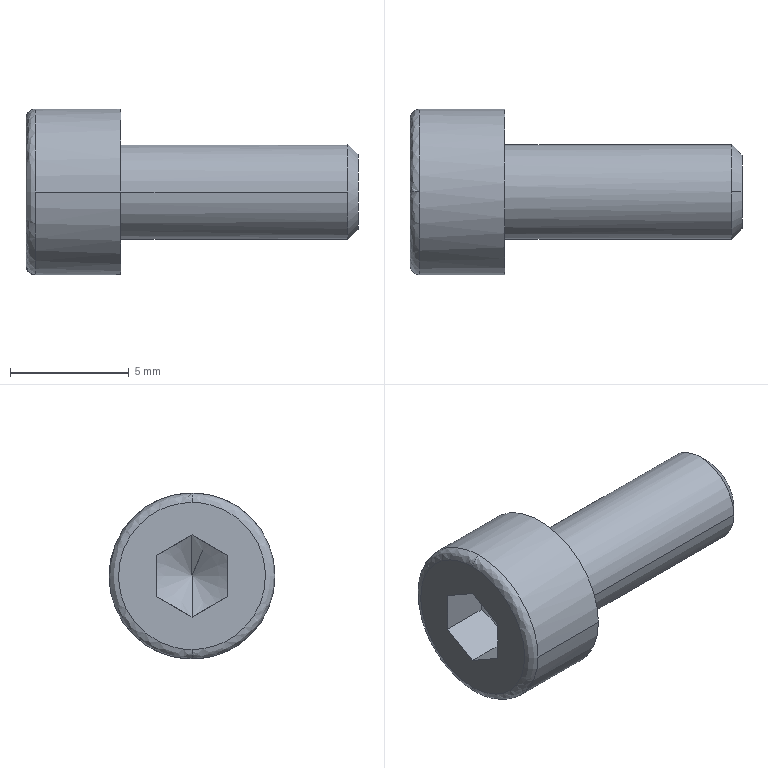Part | SolidWorks | features BaseBody 1 | 1 solid | 19 faces | box 14 x 7 x 7 mm | volume 259.154 mm3 | plane 9 | cylinder 4 | cone 4 | spline 2 | commonest cylinder face diameters 4 x2 7 x2
STEP:
#1=CARTESIAN_POINT('',(-3.6,0.,3.5));
#2=VERTEX_POINT('',#1);
#3=CARTESIAN_POINT('',(-3.6,-3.5,0.));
#4=VERTEX_POINT('',#3);
#5=CARTESIAN_POINT('',(-3.6,0.,0.));
#6=DIRECTION('',(1.,0.,0.));
#7=DIRECTION('',(0.,1.,0.));
#8=AXIS2_PLACEMENT_3D('',#5,#6,#7);
#9=CIRCLE('',#8,3.5);
#10=EDGE_CURVE('',#2,#4,#9,.T.);
#11=ORIENTED_EDGE('',*,*,#10,.F.);
#12=CARTESIAN_POINT('',(-4.,0.,3.1));
#13=VERTEX_POINT('',#12);
#14=CARTESIAN_POINT('',(-3.6,0.,3.1));
#15=DIRECTION('',(0.,-1.,0.));
#16=DIRECTION('',(0.,0.,1.));
#17=AXIS2_PLACEMENT_3D('',#14,#15,#16);
#18=CIRCLE('',#17,0.4);
#19=EDGE_CURVE('',#2,#13,#18,.T.);
#20=ORIENTED_EDGE('',*,*,#19,.T.);
#21=CARTESIAN_POINT('',(-4.,0.,-3.1));
#22=VERTEX_POINT('',#21);
#23=CARTESIAN_POINT('',(-4.,0.,3.1));
#24=CARTESIAN_POINT('',(-4.,-6.2,3.1));
#25=CARTESIAN_POINT('',(-4.,-6.2,-3.1));
#26=CARTESIAN_POINT('',(-4.,0.,-3.1));
#27=(BOUNDED_CURVE()B_SPLINE_CURVE(3,(#23,#24,#25,#26),.UNSPECIFIED.,.F.,.F.)B_SPLINE_CURVE_WITH_KNOTS((4,4),(0.25,0.75),.UNSPECIFIED.)CURVE()GEOMETRIC_REPRESENTATION_ITEM()RATIONAL_B_SPLINE_CURVE((1.,0.3333,0.3333,1.))REPRESENTATION_ITEM(''));
#28=EDGE_CURVE('',#13,#22,#27,.T.);
#29=ORIENTED_EDGE('',*,*,#28,.T.);
#30=CARTESIAN_POINT('',(-3.6,0.,-3.5));
#31=VERTEX_POINT('',#30);
#32=CARTESIAN_POINT('',(-3.6,0.,-3.1));
#33=DIRECTION('',(0.,1.,0.));
#34=DIRECTION('',(0.,0.,-1.));
#35=AXIS2_PLACEMENT_3D('',#32,#33,#34);
#36=CIRCLE('',#35,0.4);
#37=EDGE_CURVE('',#31,#22,#36,.T.);
#38=ORIENTED_EDGE('',*,*,#37,.F.);
#39=CARTESIAN_POINT('',(-3.6,0.,0.));
#40=DIRECTION('',(1.,0.,0.));
#41=DIRECTION('',(0.,1.,0.));
#42=AXIS2_PLACEMENT_3D('',#39,#40,#41);
#43=CIRCLE('',#42,3.5);
#44=EDGE_CURVE('',#4,#31,#43,.T.);
#45=ORIENTED_EDGE('',*,*,#44,.F.);
#46=EDGE_LOOP('',(#11,#20,#29,#38,#45));
#47=FACE_OUTER_BOUND('',#46,.T.);
#48=CARTESIAN_POINT('',(-3.6,0.,3.5));
#49=CARTESIAN_POINT('',(-3.6,-7.,3.5));
#50=CARTESIAN_POINT('',(-3.6,-7.,-3.5));
#51=CARTESIAN_POINT('',(-3.6,0.,-3.5));
#52=CARTESIAN_POINT('',(-3.834,0.,3.5));
#53=CARTESIAN_POINT('',(-3.834,-7.,3.5));
#54=CARTESIAN_POINT('',(-3.834,-7.,-3.5));
#55=CARTESIAN_POINT('',(-3.834,0.,-3.5));
#56=CARTESIAN_POINT('',(-4.,0.,3.334));
#57=CARTESIAN_POINT('',(-4.,-6.669,3.334));
#58=CARTESIAN_POINT('',(-4.,-6.669,-3.334));
#59=CARTESIAN_POINT('',(-4.,0.,-3.334));
#60=CARTESIAN_POINT('',(-4.,0.,3.1));
#61=CARTESIAN_POINT('',(-4.,-6.2,3.1));
#62=CARTESIAN_POINT('',(-4.,-6.2,-3.1));
#63=CARTESIAN_POINT('',(-4.,0.,-3.1));
#64=(BOUNDED_SURFACE()B_SPLINE_SURFACE(3,3,((#48,#49,#50,#51),(#52,#53,#54,#55),(#56,#57,#58,#59),(#60,#61,#62,#63)),.UNSPECIFIED.,.F.,.F.,.F.)B_SPLINE_SURFACE_WITH_KNOTS((4,4),(4,4),(0.,1.),(0.,1.),.UNSPECIFIED.)GEOMETRIC_REPRESENTATION_ITEM()RATIONAL_B_SPLINE_SURFACE(((1.,0.3333,0.3333,1.),(0.8047,0.2682,0.2682,0.8047),(0.8047,0.2682,0.2682,0.8047),(1.,0.3333,0.3333,1.)))REPRESENTATION_ITEM('')SURFACE());
#65=ADVANCED_FACE('',(#47),#64,.T.);
#66=CARTESIAN_POINT('',(0.,2.,0.));
#67=VERTEX_POINT('',#66);
#68=CARTESIAN_POINT('',(0.,-2.,0.));
#69=VERTEX_POINT('',#68);
#70=CARTESIAN_POINT('',(0.,0.,0.));
#71=DIRECTION('',(1.,0.,0.));
#72=DIRECTION('',(0.,1.,0.));
#73=AXIS2_PLACEMENT_3D('',#70,#71,#72);
#74=CIRCLE('',#73,2.);
#75=EDGE_CURVE('',#67,#69,#74,.T.);
#76=ORIENTED_EDGE('',*,*,#75,.T.);
#77=CARTESIAN_POINT('',(9.571,-2.,0.));
#78=VERTEX_POINT('',#77);
#79=CARTESIAN_POINT('',(5.875,-2.,0.));
#80=DIRECTION('',(1.,0.,0.));
#81=VECTOR('',#80,1000.);
#82=LINE('',#79,#81);
#83=EDGE_CURVE('',#69,#78,#82,.T.);
#84=ORIENTED_EDGE('',*,*,#83,.T.);
#85=CARTESIAN_POINT('',(9.571,0.,2.));
#86=VERTEX_POINT('',#85);
#87=CARTESIAN_POINT('',(9.571,0.,0.));
#88=DIRECTION('',(-1.,0.,0.));
#89=DIRECTION('',(0.,1.,0.));
#90=AXIS2_PLACEMENT_3D('',#87,#88,#89);
#91=CIRCLE('',#90,2.);
#92=EDGE_CURVE('',#78,#86,#91,.T.);
#93=ORIENTED_EDGE('',*,*,#92,.T.);
#94=CARTESIAN_POINT('',(9.571,2.,0.));
#95=VERTEX_POINT('',#94);
#96=CARTESIAN_POINT('',(9.571,0.,0.));
#97=DIRECTION('',(-1.,0.,0.));
#98=DIRECTION('',(0.,1.,0.));
#99=AXIS2_PLACEMENT_3D('',#96,#97,#98);
#100=CIRCLE('',#99,2.);
#101=EDGE_CURVE('',#86,#95,#100,.T.);
#102=ORIENTED_EDGE('',*,*,#101,.T.);
#103=CARTESIAN_POINT('',(5.875,2.,0.));
#104=DIRECTION('',(1.,0.,0.));
#105=VECTOR('',#104,1000.);
#106=LINE('',#103,#105);
#107=EDGE_CURVE('',#67,#95,#106,.T.);
#108=ORIENTED_EDGE('',*,*,#107,.F.);
#109=EDGE_LOOP('',(#76,#84,#93,#102,#108));
#110=FACE_OUTER_BOUND('',#109,.T.);
#111=CARTESIAN_POINT('',(5.875,0.,0.));
#112=DIRECTION('',(1.,0.,0.));
#113=DIRECTION('',(0.,1.,0.));
#114=AXIS2_PLACEMENT_3D('',#111,#112,#113);
#115=CYLINDRICAL_SURFACE('',#114,2.);
#116=ADVANCED_FACE('',(#110),#115,.T.);
#117=CARTESIAN_POINT('',(10.,0.,1.571));
#118=VERTEX_POINT('',#117);
#119=CARTESIAN_POINT('',(10.,0.,-1.571));
#120=VERTEX_POINT('',#119);
#121=CARTESIAN_POINT('',(10.,0.,0.));
#122=DIRECTION('',(-1.,0.,0.));
#123=DIRECTION('',(0.,0.,1.));
#124=AXIS2_PLACEMENT_3D('',#121,#122,#123);
#125=CIRCLE('',#124,1.571);
#126=EDGE_CURVE('',#118,#120,#125,.T.);
#127=ORIENTED_EDGE('',*,*,#126,.T.);
#128=CARTESIAN_POINT('',(9.571,0.,-2.));
#129=VERTEX_POINT('',#128);
#130=CARTESIAN_POINT('',(9.571,0.,-2.));
#131=DIRECTION('',(-0.7071,0.,-0.7071));
#132=VECTOR('',#131,1000.);
#133=LINE('',#130,#132);
#134=EDGE_CURVE('',#120,#129,#133,.T.);
#135=ORIENTED_EDGE('',*,*,#134,.T.);
#136=CARTESIAN_POINT('',(9.571,0.,0.));
#137=DIRECTION('',(-1.,0.,0.));
#138=DIRECTION('',(0.,1.,0.));
#139=AXIS2_PLACEMENT_3D('',#136,#137,#138);
#140=CIRCLE('',#139,2.);
#141=EDGE_CURVE('',#95,#129,#140,.T.);
#142=ORIENTED_EDGE('',*,*,#141,.F.);
#143=ORIENTED_EDGE('',*,*,#101,.F.);
#144=CARTESIAN_POINT('',(9.571,0.,2.));
#145=DIRECTION('',(-0.7071,0.,0.7071));
#146=VECTOR('',#145,1000.);
#147=LINE('',#144,#146);
#148=EDGE_CURVE('',#118,#86,#147,.T.);
#149=ORIENTED_EDGE('',*,*,#148,.F.);
#150=EDGE_LOOP('',(#127,#135,#142,#143,#149));
#151=FACE_OUTER_BOUND('',#150,.T.);
#152=CARTESIAN_POINT('',(9.571,0.,0.));
#153=DIRECTION('',(-1.,0.,0.));
#154=DIRECTION('',(0.,0.,1.));
#155=AXIS2_PLACEMENT_3D('',#152,#153,#154);
#156=CONICAL_SURFACE('',#155,2.,0.7854);
#157=ADVANCED_FACE('',(#151),#156,.T.);
#158=CARTESIAN_POINT('',(-3.6,3.5,0.));
#159=VERTEX_POINT('',#158);
#160=CARTESIAN_POINT('',(-3.6,0.,0.));
#161=DIRECTION('',(1.,0.,0.));
#162=DIRECTION('',(0.,1.,0.));
#163=AXIS2_PLACEMENT_3D('',#160,#161,#162);
#164=CIRCLE('',#163,3.5);
#165=EDGE_CURVE('',#159,#2,#164,.T.);
#166=ORIENTED_EDGE('',*,*,#165,.T.);
#167=ORIENTED_EDGE('',*,*,#10,.T.);
#168=CARTESIAN_POINT('',(0.,-3.5,0.));
#169=VERTEX_POINT('',#168);
#170=CARTESIAN_POINT('',(-2.,-3.5,0.));
#171=DIRECTION('',(1.,0.,0.));
#172=VECTOR('',#171,1000.);
#173=LINE('',#170,#172);
#174=EDGE_CURVE('',#4,#169,#173,.T.);
#175=ORIENTED_EDGE('',*,*,#174,.T.);
#176=CARTESIAN_POINT('',(0.,3.5,0.));
#177=VERTEX_POINT('',#176);
#178=CARTESIAN_POINT('',(0.,0.,0.));
#179=DIRECTION('',(1.,0.,0.));
#180=DIRECTION('',(0.,1.,0.));
#181=AXIS2_PLACEMENT_3D('',#178,#179,#180);
#182=CIRCLE('',#181,3.5);
#183=EDGE_CURVE('',#177,#169,#182,.T.);
#184=ORIENTED_EDGE('',*,*,#183,.F.);
#185=CARTESIAN_POINT('',(-2.,3.5,0.));
#186=DIRECTION('',(1.,0.,0.));
#187=VECTOR('',#186,1000.);
#188=LINE('',#185,#187);
#189=EDGE_CURVE('',#159,#177,#188,.T.);
#190=ORIENTED_EDGE('',*,*,#189,.F.);
#191=EDGE_LOOP('',(#166,#167,#175,#184,#190));
#192=FACE_OUTER_BOUND('',#191,.T.);
#193=CARTESIAN_POINT('',(-2.,0.,0.));
#194=DIRECTION('',(1.,0.,0.));
#195=DIRECTION('',(0.,1.,0.));
#196=AXIS2_PLACEMENT_3D('',#193,#194,#195);
#197=CYLINDRICAL_SURFACE('',#196,3.5);
#198=ADVANCED_FACE('',(#192),#197,.T.);
#199=CARTESIAN_POINT('',(-1.,0.,0.));
#200=VERTEX_POINT('',#199);
#201=CARTESIAN_POINT('',(-2.,0.000000012,1.732));
#202=VERTEX_POINT('',#201);
#203=CARTESIAN_POINT('',(-2.006,0.,1.742));
#204=DIRECTION('',(-0.5,0.,0.866));
#205=VECTOR('',#204,1000.);
#206=LINE('',#203,#205);
#207=EDGE_CURVE('',#200,#202,#206,.T.);
#208=ORIENTED_EDGE('',*,*,#207,.F.);
#209=CARTESIAN_POINT('',(-2.,-0.000000052,-1.732));
#210=VERTEX_POINT('',#209);
#211=CARTESIAN_POINT('',(-2.006,0.,-1.742));
#212=DIRECTION('',(-0.5,0.,-0.866));
#213=VECTOR('',#212,1000.);
#214=LINE('',#211,#213);
#215=EDGE_CURVE('',#200,#210,#214,.T.);
#216=ORIENTED_EDGE('',*,*,#215,.T.);
#217=CARTESIAN_POINT('',(-2.,-1.5,-0.866));
#218=VERTEX_POINT('',#217);
#219=CARTESIAN_POINT('',(-2.,-1.5,-0.866));
#220=CARTESIAN_POINT('',(-1.918,-1.255,-1.007));
#221=CARTESIAN_POINT('',(-1.866,-1.006,-1.151));
#222=CARTESIAN_POINT('',(-1.866,-0.4964,-1.445));
#223=CARTESIAN_POINT('',(-1.918,-0.2452,-1.59));
#224=CARTESIAN_POINT('',(-2.,-0.000000052,-1.732));
#225=B_SPLINE_CURVE_WITH_KNOTS('',3,(#219,#220,#221,#222,#223,#224),.UNSPECIFIED.,.F.,.F.,(4,2,4),(0.,0.0008746,0.001749),.UNSPECIFIED.);
#226=EDGE_CURVE('',#218,#210,#225,.T.);
#227=ORIENTED_EDGE('',*,*,#226,.F.);
#228=CARTESIAN_POINT('',(-2.,-1.5,0.866));
#229=VERTEX_POINT('',#228);
#230=CARTESIAN_POINT('',(-2.,-1.5,0.866));
#231=CARTESIAN_POINT('',(-1.918,-1.5,0.5832));
#232=CARTESIAN_POINT('',(-1.866,-1.5,0.2962));
#233=CARTESIAN_POINT('',(-1.866,-1.5,-0.2929));
#234=CARTESIAN_POINT('',(-1.918,-1.5,-0.5829));
#235=CARTESIAN_POINT('',(-2.,-1.5,-0.866));
#236=B_SPLINE_CURVE_WITH_KNOTS('',3,(#230,#231,#232,#233,#234,#235),.UNSPECIFIED.,.F.,.F.,(4,2,4),(0.,0.0008746,0.001749),.UNSPECIFIED.);
#237=EDGE_CURVE('',#229,#218,#236,.T.);
#238=ORIENTED_EDGE('',*,*,#237,.F.);
#239=CARTESIAN_POINT('',(-2.,0.000000012,1.732));
#240=CARTESIAN_POINT('',(-1.918,-0.2449,1.591));
#241=CARTESIAN_POINT('',(-1.866,-0.4935,1.447));
#242=CARTESIAN_POINT('',(-1.866,-1.004,1.153));
#243=CARTESIAN_POINT('',(-1.918,-1.255,1.008));
#244=CARTESIAN_POINT('',(-2.,-1.5,0.866));
#245=B_SPLINE_CURVE_WITH_KNOTS('',3,(#239,#240,#241,#242,#243,#244),.UNSPECIFIED.,.F.,.F.,(4,2,4),(0.,0.0008746,0.001749),.UNSPECIFIED.);
#246=EDGE_CURVE('',#202,#229,#245,.T.);
#247=ORIENTED_EDGE('',*,*,#246,.F.);
#248=EDGE_LOOP('',(#208,#216,#227,#238,#247));
#249=FACE_OUTER_BOUND('',#248,.T.);
#250=CARTESIAN_POINT('',(-2.006,0.,0.));
#251=DIRECTION('',(-1.,0.,0.));
#252=DIRECTION('',(0.,0.,1.));
#253=AXIS2_PLACEMENT_3D('',#250,#251,#252);
#254=CONICAL_SURFACE('',#253,1.742,1.047);
#255=ADVANCED_FACE('',(#249),#254,.F.);
#256=ORIENTED_EDGE('',*,*,#83,.F.);
#257=CARTESIAN_POINT('',(0.,0.,0.));
#258=DIRECTION('',(1.,0.,0.));
#259=DIRECTION('',(0.,1.,0.));
#260=AXIS2_PLACEMENT_3D('',#257,#258,#259);
#261=CIRCLE('',#260,2.);
#262=EDGE_CURVE('',#69,#67,#261,.T.);
#263=ORIENTED_EDGE('',*,*,#262,.T.);
#264=ORIENTED_EDGE('',*,*,#107,.T.);
#265=ORIENTED_EDGE('',*,*,#141,.T.);
#266=CARTESIAN_POINT('',(9.571,0.,0.));
#267=DIRECTION('',(-1.,0.,0.));
#268=DIRECTION('',(0.,1.,0.));
#269=AXIS2_PLACEMENT_3D('',#266,#267,#268);
#270=CIRCLE('',#269,2.);
#271=EDGE_CURVE('',#129,#78,#270,.T.);
#272=ORIENTED_EDGE('',*,*,#271,.T.);
#273=EDGE_LOOP('',(#256,#263,#264,#265,#272));
#274=FACE_OUTER_BOUND('',#273,.T.);
#275=CARTESIAN_POINT('',(5.875,0.,0.));
#276=DIRECTION('',(1.,0.,0.));
#277=DIRECTION('',(0.,1.,0.));
#278=AXIS2_PLACEMENT_3D('',#275,#276,#277);
#279=CYLINDRICAL_SURFACE('',#278,2.);
#280=ADVANCED_FACE('',(#274),#279,.T.);
#281=ORIENTED_EDGE('',*,*,#134,.F.);
#282=CARTESIAN_POINT('',(10.,0.,0.));
#283=DIRECTION('',(-1.,0.,0.));
#284=DIRECTION('',(0.,0.,1.));
#285=AXIS2_PLACEMENT_3D('',#282,#283,#284);
#286=CIRCLE('',#285,1.571);
#287=EDGE_CURVE('',#120,#118,#286,.T.);
#288=ORIENTED_EDGE('',*,*,#287,.T.);
#289=ORIENTED_EDGE('',*,*,#148,.T.);
#290=ORIENTED_EDGE('',*,*,#92,.F.);
#291=ORIENTED_EDGE('',*,*,#271,.F.);
#292=EDGE_LOOP('',(#281,#288,#289,#290,#291));
#293=FACE_OUTER_BOUND('',#292,.T.);
#294=CARTESIAN_POINT('',(9.571,0.,0.));
#295=DIRECTION('',(-1.,0.,0.));
#296=DIRECTION('',(0.,0.,1.));
#297=AXIS2_PLACEMENT_3D('',#294,#295,#296);
#298=CONICAL_SURFACE('',#297,2.,0.7854);
#299=ADVANCED_FACE('',(#293),#298,.T.);
#300=ORIENTED_EDGE('',*,*,#75,.F.);
#301=ORIENTED_EDGE('',*,*,#262,.F.);
#302=EDGE_LOOP('',(#300,#301));
#303=FACE_BOUND('',#302,.T.);
#304=ORIENTED_EDGE('',*,*,#183,.T.);
#305=CARTESIAN_POINT('',(0.,0.,0.));
#306=DIRECTION('',(1.,0.,0.));
#307=DIRECTION('',(0.,1.,0.));
#308=AXIS2_PLACEMENT_3D('',#305,#306,#307);
#309=CIRCLE('',#308,3.5);
#310=EDGE_CURVE('',#169,#177,#309,.T.);
#311=ORIENTED_EDGE('',*,*,#310,.T.);
#312=EDGE_LOOP('',(#304,#311));
#313=FACE_OUTER_BOUND('',#312,.T.);
#314=CARTESIAN_POINT('',(0.,2.75,0.));
#315=DIRECTION('',(1.,0.,0.));
#316=DIRECTION('',(0.,0.,-1.));
#317=AXIS2_PLACEMENT_3D('',#314,#315,#316);
#318=PLANE('',#317);
#319=ADVANCED_FACE('',(#303,#313),#318,.T.);
#320=ORIENTED_EDGE('',*,*,#126,.F.);
#321=ORIENTED_EDGE('',*,*,#287,.F.);
#322=EDGE_LOOP('',(#320,#321));
#323=FACE_OUTER_BOUND('',#322,.T.);
#324=CARTESIAN_POINT('',(10.,1.,0.));
#325=DIRECTION('',(1.,0.,0.));
#326=DIRECTION('',(0.,0.,-1.));
#327=AXIS2_PLACEMENT_3D('',#324,#325,#326);
#328=PLANE('',#327);
#329=ADVANCED_FACE('',(#323),#328,.T.);
#330=ORIENTED_EDGE('',*,*,#174,.F.);
#331=ORIENTED_EDGE('',*,*,#44,.T.);
#332=CARTESIAN_POINT('',(-3.6,0.,0.));
#333=DIRECTION('',(1.,0.,0.));
#334=DIRECTION('',(0.,1.,0.));
#335=AXIS2_PLACEMENT_3D('',#332,#333,#334);
#336=CIRCLE('',#335,3.5);
#337=EDGE_CURVE('',#31,#159,#336,.T.);
#338=ORIENTED_EDGE('',*,*,#337,.T.);
#339=ORIENTED_EDGE('',*,*,#189,.T.);
#340=ORIENTED_EDGE('',*,*,#310,.F.);
#341=EDGE_LOOP('',(#330,#331,#338,#339,#340));
#342=FACE_OUTER_BOUND('',#341,.T.);
#343=CARTESIAN_POINT('',(-2.,0.,0.));
#344=DIRECTION('',(1.,0.,0.));
#345=DIRECTION('',(0.,1.,0.));
#346=AXIS2_PLACEMENT_3D('',#343,#344,#345);
#347=CYLINDRICAL_SURFACE('',#346,3.5);
#348=ADVANCED_FACE('',(#342),#347,.T.);
#349=ORIENTED_EDGE('',*,*,#19,.F.);
#350=ORIENTED_EDGE('',*,*,#165,.F.);
#351=ORIENTED_EDGE('',*,*,#337,.F.);
#352=ORIENTED_EDGE('',*,*,#37,.T.);
#353=CARTESIAN_POINT('',(-4.,0.,-3.1));
#354=CARTESIAN_POINT('',(-4.,6.2,-3.1));
#355=CARTESIAN_POINT('',(-4.,6.2,3.1));
#356=CARTESIAN_POINT('',(-4.,0.,3.1));
#357=(BOUNDED_CURVE()B_SPLINE_CURVE(3,(#353,#354,#355,#356),.UNSPECIFIED.,.F.,.F.)B_SPLINE_CURVE_WITH_KNOTS((4,4),(0.75,1.25),.UNSPECIFIED.)CURVE()GEOMETRIC_REPRESENTATION_ITEM()RATIONAL_B_SPLINE_CURVE((1.,0.3333,0.3333,1.))REPRESENTATION_ITEM(''));
#358=EDGE_CURVE('',#22,#13,#357,.T.);
#359=ORIENTED_EDGE('',*,*,#358,.T.);
#360=EDGE_LOOP('',(#349,#350,#351,#352,#359));
#361=FACE_OUTER_BOUND('',#360,.T.);
#362=CARTESIAN_POINT('',(-3.6,0.,-3.5));
#363=CARTESIAN_POINT('',(-3.6,7.,-3.5));
#364=CARTESIAN_POINT('',(-3.6,7.,3.5));
#365=CARTESIAN_POINT('',(-3.6,0.,3.5));
#366=CARTESIAN_POINT('',(-3.834,0.,-3.5));
#367=CARTESIAN_POINT('',(-3.834,7.,-3.5));
#368=CARTESIAN_POINT('',(-3.834,7.,3.5));
#369=CARTESIAN_POINT('',(-3.834,0.,3.5));
#370=CARTESIAN_POINT('',(-4.,0.,-3.334));
#371=CARTESIAN_POINT('',(-4.,6.669,-3.334));
#372=CARTESIAN_POINT('',(-4.,6.669,3.334));
#373=CARTESIAN_POINT('',(-4.,0.,3.334));
#374=CARTESIAN_POINT('',(-4.,0.,-3.1));
#375=CARTESIAN_POINT('',(-4.,6.2,-3.1));
#376=CARTESIAN_POINT('',(-4.,6.2,3.1));
#377=CARTESIAN_POINT('',(-4.,0.,3.1));
#378=(BOUNDED_SURFACE()B_SPLINE_SURFACE(3,3,((#362,#363,#364,#365),(#366,#367,#368,#369),(#370,#371,#372,#373),(#374,#375,#376,#377)),.UNSPECIFIED.,.F.,.F.,.F.)B_SPLINE_SURFACE_WITH_KNOTS((4,4),(4,4),(0.,1.),(0.,1.),.UNSPECIFIED.)GEOMETRIC_REPRESENTATION_ITEM()RATIONAL_B_SPLINE_SURFACE(((1.,0.3333,0.3333,1.),(0.8047,0.2682,0.2682,0.8047),(0.8047,0.2682,0.2682,0.8047),(1.,0.3333,0.3333,1.)))REPRESENTATION_ITEM('')SURFACE());
#379=ADVANCED_FACE('',(#361),#378,.T.);
#380=CARTESIAN_POINT('',(-4.,-1.5,-0.866));
#381=VERTEX_POINT('',#380);
#382=CARTESIAN_POINT('',(-4.,0.,-1.732));
#383=VERTEX_POINT('',#382);
#384=CARTESIAN_POINT('',(-4.,0.,-1.732));
#385=DIRECTION('',(0.,0.866,-0.5));
#386=VECTOR('',#385,1000.);
#387=LINE('',#384,#386);
#388=EDGE_CURVE('',#381,#383,#387,.T.);
#389=ORIENTED_EDGE('',*,*,#388,.T.);
#390=CARTESIAN_POINT('',(-4.,1.5,-0.866));
#391=VERTEX_POINT('',#390);
#392=CARTESIAN_POINT('',(-4.,0.,-1.732));
#393=DIRECTION('',(0.,0.866,0.5));
#394=VECTOR('',#393,1000.);
#395=LINE('',#392,#394);
#396=EDGE_CURVE('',#383,#391,#395,.T.);
#397=ORIENTED_EDGE('',*,*,#396,.T.);
#398=CARTESIAN_POINT('',(-4.,1.5,0.866));
#399=VERTEX_POINT('',#398);
#400=CARTESIAN_POINT('',(-4.,1.5,0.866));
#401=DIRECTION('',(0.,0.,1.));
#402=VECTOR('',#401,1000.);
#403=LINE('',#400,#402);
#404=EDGE_CURVE('',#391,#399,#403,.T.);
#405=ORIENTED_EDGE('',*,*,#404,.T.);
#406=CARTESIAN_POINT('',(-4.,0.,1.732));
#407=VERTEX_POINT('',#406);
#408=CARTESIAN_POINT('',(-4.,0.,1.732));
#409=DIRECTION('',(0.,-0.866,0.5));
#410=VECTOR('',#409,1000.);
#411=LINE('',#408,#410);
#412=EDGE_CURVE('',#399,#407,#411,.T.);
#413=ORIENTED_EDGE('',*,*,#412,.T.);
#414=CARTESIAN_POINT('',(-4.,-1.5,0.866));
#415=VERTEX_POINT('',#414);
#416=CARTESIAN_POINT('',(-4.,-1.5,0.866));
#417=DIRECTION('',(0.,-0.866,-0.5));
#418=VECTOR('',#417,1000.);
#419=LINE('',#416,#418);
#420=EDGE_CURVE('',#407,#415,#419,.T.);
#421=ORIENTED_EDGE('',*,*,#420,.T.);
#422=CARTESIAN_POINT('',(-4.,-1.5,-0.866));
#423=DIRECTION('',(0.,0.,-1.));
#424=VECTOR('',#423,1000.);
#425=LINE('',#422,#424);
#426=EDGE_CURVE('',#415,#381,#425,.T.);
#427=ORIENTED_EDGE('',*,*,#426,.T.);
#428=EDGE_LOOP('',(#389,#397,#405,#413,#421,#427));
#429=FACE_BOUND('',#428,.T.);
#430=ORIENTED_EDGE('',*,*,#358,.F.);
#431=ORIENTED_EDGE('',*,*,#28,.F.);
#432=EDGE_LOOP('',(#430,#431));
#433=FACE_OUTER_BOUND('',#432,.T.);
#434=CARTESIAN_POINT('',(-4.,2.616,0.));
#435=DIRECTION('',(-1.,0.,0.));
#436=DIRECTION('',(0.,0.,1.));
#437=AXIS2_PLACEMENT_3D('',#434,#435,#436);
#438=PLANE('',#437);
#439=ADVANCED_FACE('',(#429,#433),#438,.T.);
#440=CARTESIAN_POINT('',(-2.,1.5,-0.866));
#441=VERTEX_POINT('',#440);
#442=CARTESIAN_POINT('',(-4.,1.5,-0.866));
#443=DIRECTION('',(1.,0.,0.));
#444=VECTOR('',#443,1000.);
#445=LINE('',#442,#444);
#446=EDGE_CURVE('',#391,#441,#445,.T.);
#447=ORIENTED_EDGE('',*,*,#446,.F.);
#448=ORIENTED_EDGE('',*,*,#396,.F.);
#449=CARTESIAN_POINT('',(-4.,0.,-1.732));
#450=DIRECTION('',(-1.,0.,0.));
#451=VECTOR('',#450,1000.);
#452=LINE('',#449,#451);
#453=EDGE_CURVE('',#210,#383,#452,.T.);
#454=ORIENTED_EDGE('',*,*,#453,.F.);
#455=CARTESIAN_POINT('',(-2.,1.5,-0.866));
#456=CARTESIAN_POINT('',(-1.918,1.255,-1.007));
#457=CARTESIAN_POINT('',(-1.866,1.006,-1.151));
#458=CARTESIAN_POINT('',(-1.866,0.4964,-1.445));
#459=CARTESIAN_POINT('',(-1.918,0.2452,-1.59));
#460=CARTESIAN_POINT('',(-2.,-0.000000052,-1.732));
#461=B_SPLINE_CURVE_WITH_KNOTS('',3,(#455,#456,#457,#458,#459,#460),.UNSPECIFIED.,.F.,.F.,(4,2,4),(0.,0.0008746,0.001749),.UNSPECIFIED.);
#462=EDGE_CURVE('',#441,#210,#461,.T.);
#463=ORIENTED_EDGE('',*,*,#462,.F.);
#464=EDGE_LOOP('',(#447,#448,#454,#463));
#465=FACE_OUTER_BOUND('',#464,.T.);
#466=CARTESIAN_POINT('',(-4.,1.5,-0.866));
#467=DIRECTION('',(0.,0.5,-0.866));
#468=DIRECTION('',(0.,0.866,0.5));
#469=AXIS2_PLACEMENT_3D('',#466,#467,#468);
#470=PLANE('',#469);
#471=ADVANCED_FACE('',(#465),#470,.F.);
#472=ORIENTED_EDGE('',*,*,#215,.F.);
#473=ORIENTED_EDGE('',*,*,#207,.T.);
#474=CARTESIAN_POINT('',(-2.,1.5,0.866));
#475=VERTEX_POINT('',#474);
#476=CARTESIAN_POINT('',(-2.,1.5,0.866));
#477=CARTESIAN_POINT('',(-1.918,1.255,1.007));
#478=CARTESIAN_POINT('',(-1.866,1.006,1.151));
#479=CARTESIAN_POINT('',(-1.866,0.4964,1.445));
#480=CARTESIAN_POINT('',(-1.918,0.2452,1.59));
#481=CARTESIAN_POINT('',(-2.,0.000000012,1.732));
#482=B_SPLINE_CURVE_WITH_KNOTS('',3,(#476,#477,#478,#479,#480,#481),.UNSPECIFIED.,.F.,.F.,(4,2,4),(0.,0.0008746,0.001749),.UNSPECIFIED.);
#483=EDGE_CURVE('',#475,#202,#482,.T.);
#484=ORIENTED_EDGE('',*,*,#483,.F.);
#485=CARTESIAN_POINT('',(-2.,1.5,-0.866));
#486=CARTESIAN_POINT('',(-1.918,1.5,-0.5832));
#487=CARTESIAN_POINT('',(-1.866,1.5,-0.2962));
#488=CARTESIAN_POINT('',(-1.866,1.5,0.2929));
#489=CARTESIAN_POINT('',(-1.918,1.5,0.5829));
#490=CARTESIAN_POINT('',(-2.,1.5,0.866));
#491=B_SPLINE_CURVE_WITH_KNOTS('',3,(#485,#486,#487,#488,#489,#490),.UNSPECIFIED.,.F.,.F.,(4,2,4),(0.,0.0008746,0.001749),.UNSPECIFIED.);
#492=EDGE_CURVE('',#441,#475,#491,.T.);
#493=ORIENTED_EDGE('',*,*,#492,.F.);
#494=ORIENTED_EDGE('',*,*,#462,.T.);
#495=EDGE_LOOP('',(#472,#473,#484,#493,#494));
#496=FACE_OUTER_BOUND('',#495,.T.);
#497=CARTESIAN_POINT('',(-2.006,0.,0.));
#498=DIRECTION('',(-1.,0.,0.));
#499=DIRECTION('',(0.,0.,1.));
#500=AXIS2_PLACEMENT_3D('',#497,#498,#499);
#501=CONICAL_SURFACE('',#500,1.742,1.047);
#502=ADVANCED_FACE('',(#496),#501,.F.);
#503=CARTESIAN_POINT('',(-4.,1.5,0.866));
#504=DIRECTION('',(1.,0.,0.));
#505=VECTOR('',#504,1000.);
#506=LINE('',#503,#505);
#507=EDGE_CURVE('',#399,#475,#506,.T.);
#508=ORIENTED_EDGE('',*,*,#507,.F.);
#509=ORIENTED_EDGE('',*,*,#404,.F.);
#510=ORIENTED_EDGE('',*,*,#446,.T.);
#511=ORIENTED_EDGE('',*,*,#492,.T.);
#512=EDGE_LOOP('',(#508,#509,#510,#511));
#513=FACE_OUTER_BOUND('',#512,.T.);
#514=CARTESIAN_POINT('',(-4.,1.5,0.866));
#515=DIRECTION('',(0.,1.,0.));
#516=DIRECTION('',(0.,0.,1.));
#517=AXIS2_PLACEMENT_3D('',#514,#515,#516);
#518=PLANE('',#517);
#519=ADVANCED_FACE('',(#513),#518,.F.);
#520=ORIENTED_EDGE('',*,*,#453,.T.);
#521=ORIENTED_EDGE('',*,*,#388,.F.);
#522=CARTESIAN_POINT('',(-4.,-1.5,-0.866));
#523=DIRECTION('',(-1.,0.,0.));
#524=VECTOR('',#523,1000.);
#525=LINE('',#522,#524);
#526=EDGE_CURVE('',#218,#381,#525,.T.);
#527=ORIENTED_EDGE('',*,*,#526,.F.);
#528=ORIENTED_EDGE('',*,*,#226,.T.);
#529=EDGE_LOOP('',(#520,#521,#527,#528));
#530=FACE_OUTER_BOUND('',#529,.T.);
#531=CARTESIAN_POINT('',(-4.,0.,-1.732));
#532=DIRECTION('',(0.,-0.5,-0.866));
#533=DIRECTION('',(0.,0.866,-0.5));
#534=AXIS2_PLACEMENT_3D('',#531,#532,#533);
#535=PLANE('',#534);
#536=ADVANCED_FACE('',(#530),#535,.F.);
#537=CARTESIAN_POINT('',(-4.,0.,1.732));
#538=DIRECTION('',(1.,0.,0.));
#539=VECTOR('',#538,1000.);
#540=LINE('',#537,#539);
#541=EDGE_CURVE('',#407,#202,#540,.T.);
#542=ORIENTED_EDGE('',*,*,#541,.F.);
#543=ORIENTED_EDGE('',*,*,#412,.F.);
#544=ORIENTED_EDGE('',*,*,#507,.T.);
#545=ORIENTED_EDGE('',*,*,#483,.T.);
#546=EDGE_LOOP('',(#542,#543,#544,#545));
#547=FACE_OUTER_BOUND('',#546,.T.);
#548=CARTESIAN_POINT('',(-4.,0.,1.732));
#549=DIRECTION('',(0.,0.5,0.866));
#550=DIRECTION('',(0.,-0.866,0.5));
#551=AXIS2_PLACEMENT_3D('',#548,#549,#550);
#552=PLANE('',#551);
#553=ADVANCED_FACE('',(#547),#552,.F.);
#554=ORIENTED_EDGE('',*,*,#526,.T.);
#555=ORIENTED_EDGE('',*,*,#426,.F.);
#556=CARTESIAN_POINT('',(-4.,-1.5,0.866));
#557=DIRECTION('',(-1.,0.,0.));
#558=VECTOR('',#557,1000.);
#559=LINE('',#556,#558);
#560=EDGE_CURVE('',#229,#415,#559,.T.);
#561=ORIENTED_EDGE('',*,*,#560,.F.);
#562=ORIENTED_EDGE('',*,*,#237,.T.);
#563=EDGE_LOOP('',(#554,#555,#561,#562));
#564=FACE_OUTER_BOUND('',#563,.T.);
#565=CARTESIAN_POINT('',(-4.,-1.5,-0.866));
#566=DIRECTION('',(0.,-1.,0.));
#567=DIRECTION('',(0.,0.,-1.));
#568=AXIS2_PLACEMENT_3D('',#565,#566,#567);
#569=PLANE('',#568);
#570=ADVANCED_FACE('',(#564),#569,.F.);
#571=ORIENTED_EDGE('',*,*,#560,.T.);
#572=ORIENTED_EDGE('',*,*,#420,.F.);
#573=ORIENTED_EDGE('',*,*,#541,.T.);
#574=ORIENTED_EDGE('',*,*,#246,.T.);
#575=EDGE_LOOP('',(#571,#572,#573,#574));
#576=FACE_OUTER_BOUND('',#575,.T.);
#577=CARTESIAN_POINT('',(-4.,-1.5,0.866));
#578=DIRECTION('',(0.,-0.5,0.866));
#579=DIRECTION('',(0.,-0.866,-0.5));
#580=AXIS2_PLACEMENT_3D('',#577,#578,#579);
#581=PLANE('',#580);
#582=ADVANCED_FACE('',(#576),#581,.F.);
#583=CLOSED_SHELL('',(#65,#116,#157,#198,#255,#280,#299,#319,#329,#348,#379,#439,#471,#502,#519,#536,#553,#570,#582));
#584=MANIFOLD_SOLID_BREP('',#583);
#585=CARTESIAN_POINT('',(0.,0.,0.));
#586=DIRECTION('',(0.,0.,1.));
#587=DIRECTION('',(1.,0.,0.));
#588=AXIS2_PLACEMENT_3D('',#585,#586,#587);
#589=(LENGTH_UNIT()NAMED_UNIT(*)SI_UNIT(.MILLI.,.METRE.));
#590=UNCERTAINTY_MEASURE_WITH_UNIT(LENGTH_MEASURE(0.00001),#589,'','');
#591=(NAMED_UNIT(*)PLANE_ANGLE_UNIT()SI_UNIT($,.RADIAN.));
#592=(NAMED_UNIT(*)SI_UNIT($,.STERADIAN.)SOLID_ANGLE_UNIT());
#593=(GEOMETRIC_REPRESENTATION_CONTEXT(3)GLOBAL_UNCERTAINTY_ASSIGNED_CONTEXT((#590))GLOBAL_UNIT_ASSIGNED_CONTEXT((#589,#591,#592))REPRESENTATION_CONTEXT('',''));
#594=ADVANCED_BREP_SHAPE_REPRESENTATION('',(#584,#588),#593);